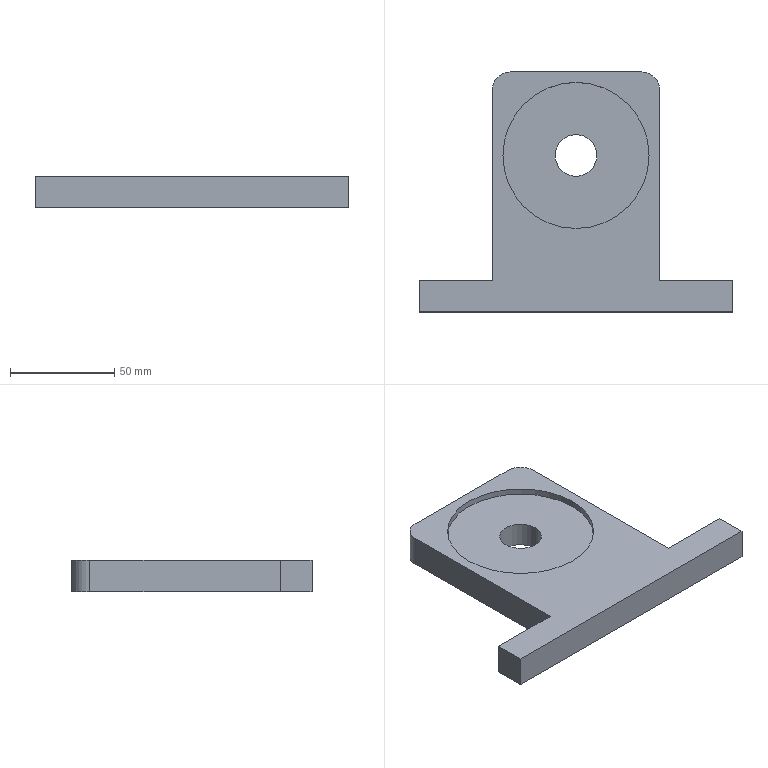Part | SolidWorks | 1 solid | 17 faces | box 150 x 115 x 15 mm | volume 137970 mm3 | plane 11 | cylinder 6 | commonest cylinder face diameters 17 x2 20 x2 70 x2
STEP:
#1=CARTESIAN_POINT('',(-10.,13.75,0.));
#2=VERTEX_POINT('',#1);
#3=CARTESIAN_POINT('',(10.,13.75,0.));
#4=VERTEX_POINT('',#3);
#5=CARTESIAN_POINT('',(0.,13.75,0.));
#6=DIRECTION('',(0.,0.,1.));
#7=DIRECTION('',(1.,0.,0.));
#8=AXIS2_PLACEMENT_3D('',#5,#6,#7);
#9=CIRCLE('',#8,10.);
#10=EDGE_CURVE('',#2,#4,#9,.T.);
#11=ORIENTED_EDGE('',*,*,#10,.F.);
#12=CARTESIAN_POINT('',(-10.,13.75,12.));
#13=VERTEX_POINT('',#12);
#14=CARTESIAN_POINT('',(-10.,13.75,-52.));
#15=DIRECTION('',(0.,0.,1.));
#16=VECTOR('',#15,1000.);
#17=LINE('',#14,#16);
#18=EDGE_CURVE('',#2,#13,#17,.T.);
#19=ORIENTED_EDGE('',*,*,#18,.T.);
#20=CARTESIAN_POINT('',(10.,13.75,12.));
#21=VERTEX_POINT('',#20);
#22=CARTESIAN_POINT('',(0.,13.75,12.));
#23=DIRECTION('',(0.,0.,1.));
#24=DIRECTION('',(1.,0.,0.));
#25=AXIS2_PLACEMENT_3D('',#22,#23,#24);
#26=CIRCLE('',#25,10.);
#27=EDGE_CURVE('',#13,#21,#26,.T.);
#28=ORIENTED_EDGE('',*,*,#27,.T.);
#29=CARTESIAN_POINT('',(10.,13.75,-52.));
#30=DIRECTION('',(0.,0.,1.));
#31=VECTOR('',#30,1000.);
#32=LINE('',#29,#31);
#33=EDGE_CURVE('',#4,#21,#32,.T.);
#34=ORIENTED_EDGE('',*,*,#33,.F.);
#35=EDGE_LOOP('',(#11,#19,#28,#34));
#36=FACE_OUTER_BOUND('',#35,.T.);
#37=CARTESIAN_POINT('',(0.,13.75,-52.));
#38=DIRECTION('',(0.,0.,1.));
#39=DIRECTION('',(1.,0.,0.));
#40=AXIS2_PLACEMENT_3D('',#37,#38,#39);
#41=CYLINDRICAL_SURFACE('',#40,10.);
#42=ADVANCED_FACE('',(#36),#41,.F.);
#43=CARTESIAN_POINT('',(-35.,13.75,12.));
#44=VERTEX_POINT('',#43);
#45=CARTESIAN_POINT('',(35.,13.75,12.));
#46=VERTEX_POINT('',#45);
#47=CARTESIAN_POINT('',(0.,13.75,12.));
#48=DIRECTION('',(0.,0.,1.));
#49=DIRECTION('',(1.,0.,0.));
#50=AXIS2_PLACEMENT_3D('',#47,#48,#49);
#51=CIRCLE('',#50,35.);
#52=EDGE_CURVE('',#44,#46,#51,.T.);
#53=ORIENTED_EDGE('',*,*,#52,.F.);
#54=CARTESIAN_POINT('',(-35.,13.75,15.));
#55=VERTEX_POINT('',#54);
#56=CARTESIAN_POINT('',(-35.,13.75,12.));
#57=DIRECTION('',(0.,0.,1.));
#58=VECTOR('',#57,1000.);
#59=LINE('',#56,#58);
#60=EDGE_CURVE('',#44,#55,#59,.T.);
#61=ORIENTED_EDGE('',*,*,#60,.T.);
#62=CARTESIAN_POINT('',(35.,13.75,15.));
#63=VERTEX_POINT('',#62);
#64=CARTESIAN_POINT('',(0.,13.75,15.));
#65=DIRECTION('',(0.,0.,1.));
#66=DIRECTION('',(1.,0.,0.));
#67=AXIS2_PLACEMENT_3D('',#64,#65,#66);
#68=CIRCLE('',#67,35.);
#69=EDGE_CURVE('',#55,#63,#68,.T.);
#70=ORIENTED_EDGE('',*,*,#69,.T.);
#71=CARTESIAN_POINT('',(35.,13.75,12.));
#72=DIRECTION('',(0.,0.,1.));
#73=VECTOR('',#72,1000.);
#74=LINE('',#71,#73);
#75=EDGE_CURVE('',#46,#63,#74,.T.);
#76=ORIENTED_EDGE('',*,*,#75,.F.);
#77=EDGE_LOOP('',(#53,#61,#70,#76));
#78=FACE_OUTER_BOUND('',#77,.T.);
#79=CARTESIAN_POINT('',(0.,13.75,12.));
#80=DIRECTION('',(0.,0.,1.));
#81=DIRECTION('',(1.,0.,0.));
#82=AXIS2_PLACEMENT_3D('',#79,#80,#81);
#83=CYLINDRICAL_SURFACE('',#82,35.);
#84=ADVANCED_FACE('',(#78),#83,.F.);
#85=CARTESIAN_POINT('',(-40.,-46.25,15.));
#86=VERTEX_POINT('',#85);
#87=CARTESIAN_POINT('',(-40.,45.25,15.));
#88=VERTEX_POINT('',#87);
#89=CARTESIAN_POINT('',(-40.,0.,15.));
#90=DIRECTION('',(0.,1.,0.));
#91=VECTOR('',#90,1000.);
#92=LINE('',#89,#91);
#93=EDGE_CURVE('',#86,#88,#92,.T.);
#94=ORIENTED_EDGE('',*,*,#93,.T.);
#95=CARTESIAN_POINT('',(-40.,45.25,0.));
#96=VERTEX_POINT('',#95);
#97=CARTESIAN_POINT('',(-40.,45.25,15.));
#98=DIRECTION('',(0.,0.,-1.));
#99=VECTOR('',#98,1000.);
#100=LINE('',#97,#99);
#101=EDGE_CURVE('',#88,#96,#100,.T.);
#102=ORIENTED_EDGE('',*,*,#101,.T.);
#103=CARTESIAN_POINT('',(-40.,-46.25,0.));
#104=VERTEX_POINT('',#103);
#105=CARTESIAN_POINT('',(-40.,0.,0.));
#106=DIRECTION('',(0.,1.,0.));
#107=VECTOR('',#106,1000.);
#108=LINE('',#105,#107);
#109=EDGE_CURVE('',#104,#96,#108,.T.);
#110=ORIENTED_EDGE('',*,*,#109,.F.);
#111=CARTESIAN_POINT('',(-40.,-46.25,15.));
#112=DIRECTION('',(0.,0.,-1.));
#113=VECTOR('',#112,1000.);
#114=LINE('',#111,#113);
#115=EDGE_CURVE('',#86,#104,#114,.T.);
#116=ORIENTED_EDGE('',*,*,#115,.F.);
#117=EDGE_LOOP('',(#94,#102,#110,#116));
#118=FACE_OUTER_BOUND('',#117,.T.);
#119=CARTESIAN_POINT('',(-40.,0.,15.));
#120=DIRECTION('',(-1.,0.,0.));
#121=DIRECTION('',(0.,0.,1.));
#122=AXIS2_PLACEMENT_3D('',#119,#120,#121);
#123=PLANE('',#122);
#124=ADVANCED_FACE('',(#118),#123,.T.);
#125=CARTESIAN_POINT('',(-75.,-46.25,0.));
#126=VERTEX_POINT('',#125);
#127=CARTESIAN_POINT('',(0.,-46.25,0.));
#128=DIRECTION('',(1.,0.,0.));
#129=VECTOR('',#128,1000.);
#130=LINE('',#127,#129);
#131=EDGE_CURVE('',#126,#104,#130,.T.);
#132=ORIENTED_EDGE('',*,*,#131,.F.);
#133=CARTESIAN_POINT('',(-75.,-46.25,15.));
#134=VERTEX_POINT('',#133);
#135=CARTESIAN_POINT('',(-75.,-46.25,15.));
#136=DIRECTION('',(0.,0.,-1.));
#137=VECTOR('',#136,1000.);
#138=LINE('',#135,#137);
#139=EDGE_CURVE('',#134,#126,#138,.T.);
#140=ORIENTED_EDGE('',*,*,#139,.F.);
#141=CARTESIAN_POINT('',(0.,-46.25,15.));
#142=DIRECTION('',(1.,0.,0.));
#143=VECTOR('',#142,1000.);
#144=LINE('',#141,#143);
#145=EDGE_CURVE('',#134,#86,#144,.T.);
#146=ORIENTED_EDGE('',*,*,#145,.T.);
#147=ORIENTED_EDGE('',*,*,#115,.T.);
#148=EDGE_LOOP('',(#132,#140,#146,#147));
#149=FACE_OUTER_BOUND('',#148,.T.);
#150=CARTESIAN_POINT('',(0.,-46.25,15.));
#151=DIRECTION('',(0.,1.,0.));
#152=DIRECTION('',(0.,0.,1.));
#153=AXIS2_PLACEMENT_3D('',#150,#151,#152);
#154=PLANE('',#153);
#155=ADVANCED_FACE('',(#149),#154,.T.);
#156=CARTESIAN_POINT('',(-75.,-61.25,0.));
#157=VERTEX_POINT('',#156);
#158=CARTESIAN_POINT('',(-75.,0.,0.));
#159=DIRECTION('',(0.,-1.,0.));
#160=VECTOR('',#159,1000.);
#161=LINE('',#158,#160);
#162=EDGE_CURVE('',#126,#157,#161,.T.);
#163=ORIENTED_EDGE('',*,*,#162,.T.);
#164=CARTESIAN_POINT('',(-75.,-61.25,15.));
#165=VERTEX_POINT('',#164);
#166=CARTESIAN_POINT('',(-75.,-61.25,15.));
#167=DIRECTION('',(0.,0.,-1.));
#168=VECTOR('',#167,1000.);
#169=LINE('',#166,#168);
#170=EDGE_CURVE('',#165,#157,#169,.T.);
#171=ORIENTED_EDGE('',*,*,#170,.F.);
#172=CARTESIAN_POINT('',(-75.,0.,15.));
#173=DIRECTION('',(0.,-1.,0.));
#174=VECTOR('',#173,1000.);
#175=LINE('',#172,#174);
#176=EDGE_CURVE('',#134,#165,#175,.T.);
#177=ORIENTED_EDGE('',*,*,#176,.F.);
#178=ORIENTED_EDGE('',*,*,#139,.T.);
#179=EDGE_LOOP('',(#163,#171,#177,#178));
#180=FACE_OUTER_BOUND('',#179,.T.);
#181=CARTESIAN_POINT('',(-75.,0.,15.));
#182=DIRECTION('',(1.,0.,0.));
#183=DIRECTION('',(0.,1.,0.));
#184=AXIS2_PLACEMENT_3D('',#181,#182,#183);
#185=PLANE('',#184);
#186=ADVANCED_FACE('',(#180),#185,.F.);
#187=CARTESIAN_POINT('',(75.,-61.25,0.));
#188=VERTEX_POINT('',#187);
#189=CARTESIAN_POINT('',(0.,-61.25,0.));
#190=DIRECTION('',(1.,0.,0.));
#191=VECTOR('',#190,1000.);
#192=LINE('',#189,#191);
#193=EDGE_CURVE('',#157,#188,#192,.T.);
#194=ORIENTED_EDGE('',*,*,#193,.T.);
#195=CARTESIAN_POINT('',(75.,-61.25,15.));
#196=VERTEX_POINT('',#195);
#197=CARTESIAN_POINT('',(75.,-61.25,15.));
#198=DIRECTION('',(0.,0.,-1.));
#199=VECTOR('',#198,1000.);
#200=LINE('',#197,#199);
#201=EDGE_CURVE('',#196,#188,#200,.T.);
#202=ORIENTED_EDGE('',*,*,#201,.F.);
#203=CARTESIAN_POINT('',(0.,-61.25,15.));
#204=DIRECTION('',(1.,0.,0.));
#205=VECTOR('',#204,1000.);
#206=LINE('',#203,#205);
#207=EDGE_CURVE('',#165,#196,#206,.T.);
#208=ORIENTED_EDGE('',*,*,#207,.F.);
#209=ORIENTED_EDGE('',*,*,#170,.T.);
#210=EDGE_LOOP('',(#194,#202,#208,#209));
#211=FACE_OUTER_BOUND('',#210,.T.);
#212=CARTESIAN_POINT('',(0.,-61.25,15.));
#213=DIRECTION('',(0.,1.,0.));
#214=DIRECTION('',(0.,0.,1.));
#215=AXIS2_PLACEMENT_3D('',#212,#213,#214);
#216=PLANE('',#215);
#217=ADVANCED_FACE('',(#211),#216,.F.);
#218=CARTESIAN_POINT('',(75.,-46.25,0.));
#219=VERTEX_POINT('',#218);
#220=CARTESIAN_POINT('',(75.,0.,0.));
#221=DIRECTION('',(0.,-1.,0.));
#222=VECTOR('',#221,1000.);
#223=LINE('',#220,#222);
#224=EDGE_CURVE('',#219,#188,#223,.T.);
#225=ORIENTED_EDGE('',*,*,#224,.F.);
#226=CARTESIAN_POINT('',(75.,-46.25,15.));
#227=VERTEX_POINT('',#226);
#228=CARTESIAN_POINT('',(75.,-46.25,15.));
#229=DIRECTION('',(0.,0.,-1.));
#230=VECTOR('',#229,1000.);
#231=LINE('',#228,#230);
#232=EDGE_CURVE('',#227,#219,#231,.T.);
#233=ORIENTED_EDGE('',*,*,#232,.F.);
#234=CARTESIAN_POINT('',(75.,0.,15.));
#235=DIRECTION('',(0.,-1.,0.));
#236=VECTOR('',#235,1000.);
#237=LINE('',#234,#236);
#238=EDGE_CURVE('',#227,#196,#237,.T.);
#239=ORIENTED_EDGE('',*,*,#238,.T.);
#240=ORIENTED_EDGE('',*,*,#201,.T.);
#241=EDGE_LOOP('',(#225,#233,#239,#240));
#242=FACE_OUTER_BOUND('',#241,.T.);
#243=CARTESIAN_POINT('',(75.,0.,15.));
#244=DIRECTION('',(1.,0.,0.));
#245=DIRECTION('',(0.,1.,0.));
#246=AXIS2_PLACEMENT_3D('',#243,#244,#245);
#247=PLANE('',#246);
#248=ADVANCED_FACE('',(#242),#247,.T.);
#249=CARTESIAN_POINT('',(40.,-46.25,0.));
#250=VERTEX_POINT('',#249);
#251=CARTESIAN_POINT('',(0.,-46.25,0.));
#252=DIRECTION('',(1.,0.,0.));
#253=VECTOR('',#252,1000.);
#254=LINE('',#251,#253);
#255=EDGE_CURVE('',#250,#219,#254,.T.);
#256=ORIENTED_EDGE('',*,*,#255,.F.);
#257=CARTESIAN_POINT('',(40.,-46.25,15.));
#258=VERTEX_POINT('',#257);
#259=CARTESIAN_POINT('',(40.,-46.25,15.));
#260=DIRECTION('',(0.,0.,-1.));
#261=VECTOR('',#260,1000.);
#262=LINE('',#259,#261);
#263=EDGE_CURVE('',#258,#250,#262,.T.);
#264=ORIENTED_EDGE('',*,*,#263,.F.);
#265=CARTESIAN_POINT('',(0.,-46.25,15.));
#266=DIRECTION('',(1.,0.,0.));
#267=VECTOR('',#266,1000.);
#268=LINE('',#265,#267);
#269=EDGE_CURVE('',#258,#227,#268,.T.);
#270=ORIENTED_EDGE('',*,*,#269,.T.);
#271=ORIENTED_EDGE('',*,*,#232,.T.);
#272=EDGE_LOOP('',(#256,#264,#270,#271));
#273=FACE_OUTER_BOUND('',#272,.T.);
#274=CARTESIAN_POINT('',(0.,-46.25,15.));
#275=DIRECTION('',(0.,1.,0.));
#276=DIRECTION('',(0.,0.,1.));
#277=AXIS2_PLACEMENT_3D('',#274,#275,#276);
#278=PLANE('',#277);
#279=ADVANCED_FACE('',(#273),#278,.T.);
#280=CARTESIAN_POINT('',(40.,45.25,0.));
#281=VERTEX_POINT('',#280);
#282=CARTESIAN_POINT('',(40.,0.,0.));
#283=DIRECTION('',(0.,1.,0.));
#284=VECTOR('',#283,1000.);
#285=LINE('',#282,#284);
#286=EDGE_CURVE('',#250,#281,#285,.T.);
#287=ORIENTED_EDGE('',*,*,#286,.T.);
#288=CARTESIAN_POINT('',(40.,45.25,15.));
#289=VERTEX_POINT('',#288);
#290=CARTESIAN_POINT('',(40.,45.25,15.));
#291=DIRECTION('',(0.,0.,1.));
#292=VECTOR('',#291,1000.);
#293=LINE('',#290,#292);
#294=EDGE_CURVE('',#281,#289,#293,.T.);
#295=ORIENTED_EDGE('',*,*,#294,.T.);
#296=CARTESIAN_POINT('',(40.,0.,15.));
#297=DIRECTION('',(0.,1.,0.));
#298=VECTOR('',#297,1000.);
#299=LINE('',#296,#298);
#300=EDGE_CURVE('',#258,#289,#299,.T.);
#301=ORIENTED_EDGE('',*,*,#300,.F.);
#302=ORIENTED_EDGE('',*,*,#263,.T.);
#303=EDGE_LOOP('',(#287,#295,#301,#302));
#304=FACE_OUTER_BOUND('',#303,.T.);
#305=CARTESIAN_POINT('',(40.,0.,15.));
#306=DIRECTION('',(-1.,0.,0.));
#307=DIRECTION('',(0.,-1.,0.));
#308=AXIS2_PLACEMENT_3D('',#305,#306,#307);
#309=PLANE('',#308);
#310=ADVANCED_FACE('',(#304),#309,.F.);
#311=CARTESIAN_POINT('',(-31.5,53.75,15.));
#312=VERTEX_POINT('',#311);
#313=CARTESIAN_POINT('',(31.5,53.75,15.));
#314=VERTEX_POINT('',#313);
#315=CARTESIAN_POINT('',(0.,53.75,15.));
#316=DIRECTION('',(1.,0.,0.));
#317=VECTOR('',#316,1000.);
#318=LINE('',#315,#317);
#319=EDGE_CURVE('',#312,#314,#318,.T.);
#320=ORIENTED_EDGE('',*,*,#319,.T.);
#321=CARTESIAN_POINT('',(31.5,53.75,0.));
#322=VERTEX_POINT('',#321);
#323=CARTESIAN_POINT('',(31.5,53.75,0.));
#324=DIRECTION('',(0.,0.,-1.));
#325=VECTOR('',#324,1000.);
#326=LINE('',#323,#325);
#327=EDGE_CURVE('',#314,#322,#326,.T.);
#328=ORIENTED_EDGE('',*,*,#327,.T.);
#329=CARTESIAN_POINT('',(-31.5,53.75,0.));
#330=VERTEX_POINT('',#329);
#331=CARTESIAN_POINT('',(0.,53.75,0.));
#332=DIRECTION('',(1.,0.,0.));
#333=VECTOR('',#332,1000.);
#334=LINE('',#331,#333);
#335=EDGE_CURVE('',#330,#322,#334,.T.);
#336=ORIENTED_EDGE('',*,*,#335,.F.);
#337=CARTESIAN_POINT('',(-31.5,53.75,15.));
#338=DIRECTION('',(0.,0.,1.));
#339=VECTOR('',#338,1000.);
#340=LINE('',#337,#339);
#341=EDGE_CURVE('',#330,#312,#340,.T.);
#342=ORIENTED_EDGE('',*,*,#341,.T.);
#343=EDGE_LOOP('',(#320,#328,#336,#342));
#344=FACE_OUTER_BOUND('',#343,.T.);
#345=CARTESIAN_POINT('',(0.,53.75,15.));
#346=DIRECTION('',(0.,1.,0.));
#347=DIRECTION('',(-1.,0.,0.));
#348=AXIS2_PLACEMENT_3D('',#345,#346,#347);
#349=PLANE('',#348);
#350=ADVANCED_FACE('',(#344),#349,.T.);
#351=CARTESIAN_POINT('',(0.,13.75,15.));
#352=DIRECTION('',(0.,0.,1.));
#353=DIRECTION('',(1.,0.,0.));
#354=AXIS2_PLACEMENT_3D('',#351,#352,#353);
#355=CIRCLE('',#354,35.);
#356=EDGE_CURVE('',#63,#55,#355,.T.);
#357=ORIENTED_EDGE('',*,*,#356,.F.);
#358=ORIENTED_EDGE('',*,*,#69,.F.);
#359=EDGE_LOOP('',(#357,#358));
#360=FACE_BOUND('',#359,.T.);
#361=ORIENTED_EDGE('',*,*,#300,.T.);
#362=CARTESIAN_POINT('',(31.5,45.25,15.));
#363=DIRECTION('',(0.,0.,1.));
#364=DIRECTION('',(1.,0.,0.));
#365=AXIS2_PLACEMENT_3D('',#362,#363,#364);
#366=CIRCLE('',#365,8.5);
#367=EDGE_CURVE('',#289,#314,#366,.T.);
#368=ORIENTED_EDGE('',*,*,#367,.T.);
#369=ORIENTED_EDGE('',*,*,#319,.F.);
#370=CARTESIAN_POINT('',(-31.5,45.25,15.));
#371=DIRECTION('',(0.,0.,1.));
#372=DIRECTION('',(1.,0.,0.));
#373=AXIS2_PLACEMENT_3D('',#370,#371,#372);
#374=CIRCLE('',#373,8.5);
#375=EDGE_CURVE('',#312,#88,#374,.T.);
#376=ORIENTED_EDGE('',*,*,#375,.T.);
#377=ORIENTED_EDGE('',*,*,#93,.F.);
#378=ORIENTED_EDGE('',*,*,#145,.F.);
#379=ORIENTED_EDGE('',*,*,#176,.T.);
#380=ORIENTED_EDGE('',*,*,#207,.T.);
#381=ORIENTED_EDGE('',*,*,#238,.F.);
#382=ORIENTED_EDGE('',*,*,#269,.F.);
#383=EDGE_LOOP('',(#361,#368,#369,#376,#377,#378,#379,#380,#381,#382));
#384=FACE_OUTER_BOUND('',#383,.T.);
#385=CARTESIAN_POINT('',(0.,0.,15.));
#386=DIRECTION('',(0.,0.,1.));
#387=DIRECTION('',(1.,0.,0.));
#388=AXIS2_PLACEMENT_3D('',#385,#386,#387);
#389=PLANE('',#388);
#390=ADVANCED_FACE('',(#360,#384),#389,.T.);
#391=CARTESIAN_POINT('',(0.,13.75,0.));
#392=DIRECTION('',(0.,0.,1.));
#393=DIRECTION('',(1.,0.,0.));
#394=AXIS2_PLACEMENT_3D('',#391,#392,#393);
#395=CIRCLE('',#394,10.);
#396=EDGE_CURVE('',#4,#2,#395,.T.);
#397=ORIENTED_EDGE('',*,*,#396,.T.);
#398=ORIENTED_EDGE('',*,*,#10,.T.);
#399=EDGE_LOOP('',(#397,#398));
#400=FACE_BOUND('',#399,.T.);
#401=ORIENTED_EDGE('',*,*,#335,.T.);
#402=CARTESIAN_POINT('',(31.5,45.25,0.));
#403=DIRECTION('',(0.,0.,-1.));
#404=DIRECTION('',(1.,0.,0.));
#405=AXIS2_PLACEMENT_3D('',#402,#403,#404);
#406=CIRCLE('',#405,8.5);
#407=EDGE_CURVE('',#322,#281,#406,.T.);
#408=ORIENTED_EDGE('',*,*,#407,.T.);
#409=ORIENTED_EDGE('',*,*,#286,.F.);
#410=ORIENTED_EDGE('',*,*,#255,.T.);
#411=ORIENTED_EDGE('',*,*,#224,.T.);
#412=ORIENTED_EDGE('',*,*,#193,.F.);
#413=ORIENTED_EDGE('',*,*,#162,.F.);
#414=ORIENTED_EDGE('',*,*,#131,.T.);
#415=ORIENTED_EDGE('',*,*,#109,.T.);
#416=CARTESIAN_POINT('',(-31.5,45.25,0.));
#417=DIRECTION('',(0.,0.,-1.));
#418=DIRECTION('',(1.,0.,0.));
#419=AXIS2_PLACEMENT_3D('',#416,#417,#418);
#420=CIRCLE('',#419,8.5);
#421=EDGE_CURVE('',#96,#330,#420,.T.);
#422=ORIENTED_EDGE('',*,*,#421,.T.);
#423=EDGE_LOOP('',(#401,#408,#409,#410,#411,#412,#413,#414,#415,#422));
#424=FACE_OUTER_BOUND('',#423,.T.);
#425=CARTESIAN_POINT('',(0.,0.,0.));
#426=DIRECTION('',(0.,0.,1.));
#427=DIRECTION('',(1.,0.,0.));
#428=AXIS2_PLACEMENT_3D('',#425,#426,#427);
#429=PLANE('',#428);
#430=ADVANCED_FACE('',(#400,#424),#429,.F.);
#431=ORIENTED_EDGE('',*,*,#367,.F.);
#432=ORIENTED_EDGE('',*,*,#294,.F.);
#433=ORIENTED_EDGE('',*,*,#407,.F.);
#434=ORIENTED_EDGE('',*,*,#327,.F.);
#435=EDGE_LOOP('',(#431,#432,#433,#434));
#436=FACE_OUTER_BOUND('',#435,.T.);
#437=CARTESIAN_POINT('',(31.5,45.25,15.));
#438=DIRECTION('',(0.,0.,1.));
#439=DIRECTION('',(1.,0.,0.));
#440=AXIS2_PLACEMENT_3D('',#437,#438,#439);
#441=CYLINDRICAL_SURFACE('',#440,8.5);
#442=ADVANCED_FACE('',(#436),#441,.T.);
#443=ORIENTED_EDGE('',*,*,#375,.F.);
#444=ORIENTED_EDGE('',*,*,#341,.F.);
#445=ORIENTED_EDGE('',*,*,#421,.F.);
#446=ORIENTED_EDGE('',*,*,#101,.F.);
#447=EDGE_LOOP('',(#443,#444,#445,#446));
#448=FACE_OUTER_BOUND('',#447,.T.);
#449=CARTESIAN_POINT('',(-31.5,45.25,15.));
#450=DIRECTION('',(0.,0.,-1.));
#451=DIRECTION('',(-1.,0.,0.));
#452=AXIS2_PLACEMENT_3D('',#449,#450,#451);
#453=CYLINDRICAL_SURFACE('',#452,8.5);
#454=ADVANCED_FACE('',(#448),#453,.T.);
#455=ORIENTED_EDGE('',*,*,#60,.F.);
#456=CARTESIAN_POINT('',(0.,13.75,12.));
#457=DIRECTION('',(0.,0.,1.));
#458=DIRECTION('',(1.,0.,0.));
#459=AXIS2_PLACEMENT_3D('',#456,#457,#458);
#460=CIRCLE('',#459,35.);
#461=EDGE_CURVE('',#46,#44,#460,.T.);
#462=ORIENTED_EDGE('',*,*,#461,.F.);
#463=ORIENTED_EDGE('',*,*,#75,.T.);
#464=ORIENTED_EDGE('',*,*,#356,.T.);
#465=EDGE_LOOP('',(#455,#462,#463,#464));
#466=FACE_OUTER_BOUND('',#465,.T.);
#467=CARTESIAN_POINT('',(0.,13.75,12.));
#468=DIRECTION('',(0.,0.,1.));
#469=DIRECTION('',(1.,0.,0.));
#470=AXIS2_PLACEMENT_3D('',#467,#468,#469);
#471=CYLINDRICAL_SURFACE('',#470,35.);
#472=ADVANCED_FACE('',(#466),#471,.F.);
#473=CARTESIAN_POINT('',(0.,13.75,12.));
#474=DIRECTION('',(0.,0.,1.));
#475=DIRECTION('',(1.,0.,0.));
#476=AXIS2_PLACEMENT_3D('',#473,#474,#475);
#477=CIRCLE('',#476,10.);
#478=EDGE_CURVE('',#21,#13,#477,.T.);
#479=ORIENTED_EDGE('',*,*,#478,.F.);
#480=ORIENTED_EDGE('',*,*,#27,.F.);
#481=EDGE_LOOP('',(#479,#480));
#482=FACE_BOUND('',#481,.T.);
#483=ORIENTED_EDGE('',*,*,#461,.T.);
#484=ORIENTED_EDGE('',*,*,#52,.T.);
#485=EDGE_LOOP('',(#483,#484));
#486=FACE_OUTER_BOUND('',#485,.T.);
#487=CARTESIAN_POINT('',(0.,13.75,12.));
#488=DIRECTION('',(0.,0.,1.));
#489=DIRECTION('',(1.,0.,0.));
#490=AXIS2_PLACEMENT_3D('',#487,#488,#489);
#491=PLANE('',#490);
#492=ADVANCED_FACE('',(#482,#486),#491,.T.);
#493=ORIENTED_EDGE('',*,*,#18,.F.);
#494=ORIENTED_EDGE('',*,*,#396,.F.);
#495=ORIENTED_EDGE('',*,*,#33,.T.);
#496=ORIENTED_EDGE('',*,*,#478,.T.);
#497=EDGE_LOOP('',(#493,#494,#495,#496));
#498=FACE_OUTER_BOUND('',#497,.T.);
#499=CARTESIAN_POINT('',(0.,13.75,-52.));
#500=DIRECTION('',(0.,0.,1.));
#501=DIRECTION('',(1.,0.,0.));
#502=AXIS2_PLACEMENT_3D('',#499,#500,#501);
#503=CYLINDRICAL_SURFACE('',#502,10.);
#504=ADVANCED_FACE('',(#498),#503,.F.);
#505=CLOSED_SHELL('',(#42,#84,#124,#155,#186,#217,#248,#279,#310,#350,#390,#430,#442,#454,#472,#492,#504));
#506=MANIFOLD_SOLID_BREP('',#505);
#507=CARTESIAN_POINT('',(0.,0.,0.));
#508=DIRECTION('',(0.,0.,1.));
#509=DIRECTION('',(1.,0.,0.));
#510=AXIS2_PLACEMENT_3D('',#507,#508,#509);
#511=(LENGTH_UNIT()NAMED_UNIT(*)SI_UNIT(.MILLI.,.METRE.));
#512=UNCERTAINTY_MEASURE_WITH_UNIT(LENGTH_MEASURE(0.00001),#511,'','');
#513=(NAMED_UNIT(*)PLANE_ANGLE_UNIT()SI_UNIT($,.RADIAN.));
#514=(NAMED_UNIT(*)SI_UNIT($,.STERADIAN.)SOLID_ANGLE_UNIT());
#515=(GEOMETRIC_REPRESENTATION_CONTEXT(3)GLOBAL_UNCERTAINTY_ASSIGNED_CONTEXT((#512))GLOBAL_UNIT_ASSIGNED_CONTEXT((#511,#513,#514))REPRESENTATION_CONTEXT('',''));
#516=ADVANCED_BREP_SHAPE_REPRESENTATION('',(#506,#510),#515);